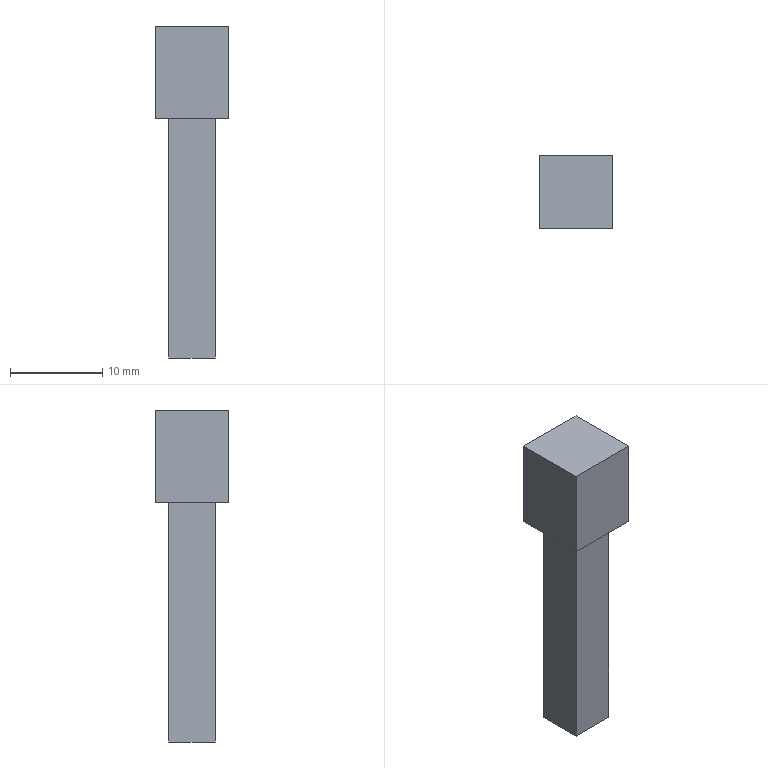Part | NX | features DATUM_CSYS 3, EXTRUDE 2, SKETCH 2 | 1 solid | 11 faces | box 8 x 8 x 36 mm | volume 1290 mm3 | plane 11
STEP:
#1=CARTESIAN_POINT('',(0.,5.,0.));
#2=VERTEX_POINT('',#1);
#3=CARTESIAN_POINT('',(0.,0.,0.));
#4=VERTEX_POINT('',#3);
#5=CARTESIAN_POINT('',(0.,5.,0.));
#6=DIRECTION('',(0.,-1.,0.));
#7=VECTOR('',#6,1000.);
#8=LINE('',#5,#7);
#9=EDGE_CURVE('',#2,#4,#8,.T.);
#10=ORIENTED_EDGE('',*,*,#9,.T.);
#11=CARTESIAN_POINT('',(0.,0.,26.));
#12=VERTEX_POINT('',#11);
#13=CARTESIAN_POINT('',(0.,0.,26.));
#14=DIRECTION('',(0.,0.,-1.));
#15=VECTOR('',#14,1000.);
#16=LINE('',#13,#15);
#17=EDGE_CURVE('',#12,#4,#16,.T.);
#18=ORIENTED_EDGE('',*,*,#17,.F.);
#19=CARTESIAN_POINT('',(0.,5.,26.));
#20=VERTEX_POINT('',#19);
#21=CARTESIAN_POINT('',(0.,5.,26.));
#22=DIRECTION('',(0.,-1.,0.));
#23=VECTOR('',#22,1000.);
#24=LINE('',#21,#23);
#25=EDGE_CURVE('',#20,#12,#24,.T.);
#26=ORIENTED_EDGE('',*,*,#25,.F.);
#27=CARTESIAN_POINT('',(0.,5.,26.));
#28=DIRECTION('',(0.,0.,-1.));
#29=VECTOR('',#28,1000.);
#30=LINE('',#27,#29);
#31=EDGE_CURVE('',#20,#2,#30,.T.);
#32=ORIENTED_EDGE('',*,*,#31,.T.);
#33=EDGE_LOOP('',(#10,#18,#26,#32));
#34=FACE_BOUND('',#33,.T.);
#35=CARTESIAN_POINT('',(0.,5.,26.));
#36=DIRECTION('',(1.,0.,0.));
#37=DIRECTION('',(0.,1.,0.));
#38=AXIS2_PLACEMENT_3D('',#35,#36,#37);
#39=PLANE('',#38);
#40=ADVANCED_FACE('',(#34),#39,.F.);
#41=CARTESIAN_POINT('',(5.,0.,0.));
#42=VERTEX_POINT('',#41);
#43=CARTESIAN_POINT('',(0.,0.,0.));
#44=DIRECTION('',(1.,0.,0.));
#45=VECTOR('',#44,1000.);
#46=LINE('',#43,#45);
#47=EDGE_CURVE('',#4,#42,#46,.T.);
#48=ORIENTED_EDGE('',*,*,#47,.T.);
#49=CARTESIAN_POINT('',(5.,0.,26.));
#50=VERTEX_POINT('',#49);
#51=CARTESIAN_POINT('',(5.,0.,26.));
#52=DIRECTION('',(0.,0.,-1.));
#53=VECTOR('',#52,1000.);
#54=LINE('',#51,#53);
#55=EDGE_CURVE('',#50,#42,#54,.T.);
#56=ORIENTED_EDGE('',*,*,#55,.F.);
#57=CARTESIAN_POINT('',(0.,0.,26.));
#58=DIRECTION('',(1.,0.,0.));
#59=VECTOR('',#58,1000.);
#60=LINE('',#57,#59);
#61=EDGE_CURVE('',#12,#50,#60,.T.);
#62=ORIENTED_EDGE('',*,*,#61,.F.);
#63=ORIENTED_EDGE('',*,*,#17,.T.);
#64=EDGE_LOOP('',(#48,#56,#62,#63));
#65=FACE_BOUND('',#64,.T.);
#66=CARTESIAN_POINT('',(0.,0.,26.));
#67=DIRECTION('',(0.,1.,0.));
#68=DIRECTION('',(0.,0.,1.));
#69=AXIS2_PLACEMENT_3D('',#66,#67,#68);
#70=PLANE('',#69);
#71=ADVANCED_FACE('',(#65),#70,.F.);
#72=CARTESIAN_POINT('',(5.,5.,0.));
#73=VERTEX_POINT('',#72);
#74=CARTESIAN_POINT('',(5.,0.,0.));
#75=DIRECTION('',(0.,1.,0.));
#76=VECTOR('',#75,1000.);
#77=LINE('',#74,#76);
#78=EDGE_CURVE('',#42,#73,#77,.T.);
#79=ORIENTED_EDGE('',*,*,#78,.T.);
#80=CARTESIAN_POINT('',(5.,5.,26.));
#81=VERTEX_POINT('',#80);
#82=CARTESIAN_POINT('',(5.,5.,26.));
#83=DIRECTION('',(0.,0.,-1.));
#84=VECTOR('',#83,1000.);
#85=LINE('',#82,#84);
#86=EDGE_CURVE('',#81,#73,#85,.T.);
#87=ORIENTED_EDGE('',*,*,#86,.F.);
#88=CARTESIAN_POINT('',(5.,0.,26.));
#89=DIRECTION('',(0.,1.,0.));
#90=VECTOR('',#89,1000.);
#91=LINE('',#88,#90);
#92=EDGE_CURVE('',#50,#81,#91,.T.);
#93=ORIENTED_EDGE('',*,*,#92,.F.);
#94=ORIENTED_EDGE('',*,*,#55,.T.);
#95=EDGE_LOOP('',(#79,#87,#93,#94));
#96=FACE_BOUND('',#95,.T.);
#97=CARTESIAN_POINT('',(5.,0.,26.));
#98=DIRECTION('',(-1.,0.,0.));
#99=DIRECTION('',(0.,0.,1.));
#100=AXIS2_PLACEMENT_3D('',#97,#98,#99);
#101=PLANE('',#100);
#102=ADVANCED_FACE('',(#96),#101,.F.);
#103=CARTESIAN_POINT('',(5.,5.,0.));
#104=DIRECTION('',(-1.,0.,0.));
#105=VECTOR('',#104,1000.);
#106=LINE('',#103,#105);
#107=EDGE_CURVE('',#73,#2,#106,.T.);
#108=ORIENTED_EDGE('',*,*,#107,.T.);
#109=ORIENTED_EDGE('',*,*,#31,.F.);
#110=CARTESIAN_POINT('',(5.,5.,26.));
#111=DIRECTION('',(-1.,0.,0.));
#112=VECTOR('',#111,1000.);
#113=LINE('',#110,#112);
#114=EDGE_CURVE('',#81,#20,#113,.T.);
#115=ORIENTED_EDGE('',*,*,#114,.F.);
#116=ORIENTED_EDGE('',*,*,#86,.T.);
#117=EDGE_LOOP('',(#108,#109,#115,#116));
#118=FACE_BOUND('',#117,.T.);
#119=CARTESIAN_POINT('',(5.,5.,26.));
#120=DIRECTION('',(0.,-1.,0.));
#121=DIRECTION('',(0.,0.,-1.));
#122=AXIS2_PLACEMENT_3D('',#119,#120,#121);
#123=PLANE('',#122);
#124=ADVANCED_FACE('',(#118),#123,.F.);
#125=ORIENTED_EDGE('',*,*,#9,.F.);
#126=ORIENTED_EDGE('',*,*,#107,.F.);
#127=ORIENTED_EDGE('',*,*,#78,.F.);
#128=ORIENTED_EDGE('',*,*,#47,.F.);
#129=EDGE_LOOP('',(#125,#126,#127,#128));
#130=FACE_BOUND('',#129,.T.);
#131=CARTESIAN_POINT('',(0.,0.,0.));
#132=DIRECTION('',(0.,0.,1.));
#133=DIRECTION('',(1.,0.,0.));
#134=AXIS2_PLACEMENT_3D('',#131,#132,#133);
#135=PLANE('',#134);
#136=ADVANCED_FACE('',(#130),#135,.F.);
#137=CARTESIAN_POINT('',(-1.5,6.5,26.));
#138=VERTEX_POINT('',#137);
#139=CARTESIAN_POINT('',(-1.5,-1.5,26.));
#140=VERTEX_POINT('',#139);
#141=CARTESIAN_POINT('',(-1.5,6.5,26.));
#142=DIRECTION('',(0.,-1.,0.));
#143=VECTOR('',#142,1000.);
#144=LINE('',#141,#143);
#145=EDGE_CURVE('',#138,#140,#144,.T.);
#146=ORIENTED_EDGE('',*,*,#145,.F.);
#147=CARTESIAN_POINT('',(6.5,6.5,26.));
#148=VERTEX_POINT('',#147);
#149=CARTESIAN_POINT('',(6.5,6.5,26.));
#150=DIRECTION('',(-1.,0.,0.));
#151=VECTOR('',#150,1000.);
#152=LINE('',#149,#151);
#153=EDGE_CURVE('',#148,#138,#152,.T.);
#154=ORIENTED_EDGE('',*,*,#153,.F.);
#155=CARTESIAN_POINT('',(6.5,-1.5,26.));
#156=VERTEX_POINT('',#155);
#157=CARTESIAN_POINT('',(6.5,-1.5,26.));
#158=DIRECTION('',(0.,1.,0.));
#159=VECTOR('',#158,1000.);
#160=LINE('',#157,#159);
#161=EDGE_CURVE('',#156,#148,#160,.T.);
#162=ORIENTED_EDGE('',*,*,#161,.F.);
#163=CARTESIAN_POINT('',(-1.5,-1.5,26.));
#164=DIRECTION('',(1.,0.,0.));
#165=VECTOR('',#164,1000.);
#166=LINE('',#163,#165);
#167=EDGE_CURVE('',#140,#156,#166,.T.);
#168=ORIENTED_EDGE('',*,*,#167,.F.);
#169=EDGE_LOOP('',(#146,#154,#162,#168));
#170=FACE_BOUND('',#169,.T.);
#171=ORIENTED_EDGE('',*,*,#114,.T.);
#172=ORIENTED_EDGE('',*,*,#25,.T.);
#173=ORIENTED_EDGE('',*,*,#61,.T.);
#174=ORIENTED_EDGE('',*,*,#92,.T.);
#175=EDGE_LOOP('',(#171,#172,#173,#174));
#176=FACE_BOUND('',#175,.T.);
#177=CARTESIAN_POINT('',(0.,0.,26.));
#178=DIRECTION('',(0.,0.,1.));
#179=DIRECTION('',(1.,0.,0.));
#180=AXIS2_PLACEMENT_3D('',#177,#178,#179);
#181=PLANE('',#180);
#182=ADVANCED_FACE('',(#170,#176),#181,.F.);
#183=ORIENTED_EDGE('',*,*,#145,.T.);
#184=CARTESIAN_POINT('',(-1.5,-1.5,36.));
#185=VERTEX_POINT('',#184);
#186=CARTESIAN_POINT('',(-1.5,-1.5,36.));
#187=DIRECTION('',(0.,0.,-1.));
#188=VECTOR('',#187,1000.);
#189=LINE('',#186,#188);
#190=EDGE_CURVE('',#185,#140,#189,.T.);
#191=ORIENTED_EDGE('',*,*,#190,.F.);
#192=CARTESIAN_POINT('',(-1.5,6.5,36.));
#193=VERTEX_POINT('',#192);
#194=CARTESIAN_POINT('',(-1.5,6.5,36.));
#195=DIRECTION('',(0.,-1.,0.));
#196=VECTOR('',#195,1000.);
#197=LINE('',#194,#196);
#198=EDGE_CURVE('',#193,#185,#197,.T.);
#199=ORIENTED_EDGE('',*,*,#198,.F.);
#200=CARTESIAN_POINT('',(-1.5,6.5,36.));
#201=DIRECTION('',(0.,0.,-1.));
#202=VECTOR('',#201,1000.);
#203=LINE('',#200,#202);
#204=EDGE_CURVE('',#193,#138,#203,.T.);
#205=ORIENTED_EDGE('',*,*,#204,.T.);
#206=EDGE_LOOP('',(#183,#191,#199,#205));
#207=FACE_BOUND('',#206,.T.);
#208=CARTESIAN_POINT('',(-1.5,6.5,36.));
#209=DIRECTION('',(1.,0.,0.));
#210=DIRECTION('',(0.,0.,-1.));
#211=AXIS2_PLACEMENT_3D('',#208,#209,#210);
#212=PLANE('',#211);
#213=ADVANCED_FACE('',(#207),#212,.F.);
#214=ORIENTED_EDGE('',*,*,#167,.T.);
#215=CARTESIAN_POINT('',(6.5,-1.5,36.));
#216=VERTEX_POINT('',#215);
#217=CARTESIAN_POINT('',(6.5,-1.5,36.));
#218=DIRECTION('',(0.,0.,-1.));
#219=VECTOR('',#218,1000.);
#220=LINE('',#217,#219);
#221=EDGE_CURVE('',#216,#156,#220,.T.);
#222=ORIENTED_EDGE('',*,*,#221,.F.);
#223=CARTESIAN_POINT('',(-1.5,-1.5,36.));
#224=DIRECTION('',(1.,0.,0.));
#225=VECTOR('',#224,1000.);
#226=LINE('',#223,#225);
#227=EDGE_CURVE('',#185,#216,#226,.T.);
#228=ORIENTED_EDGE('',*,*,#227,.F.);
#229=ORIENTED_EDGE('',*,*,#190,.T.);
#230=EDGE_LOOP('',(#214,#222,#228,#229));
#231=FACE_BOUND('',#230,.T.);
#232=CARTESIAN_POINT('',(-1.5,-1.5,36.));
#233=DIRECTION('',(0.,1.,0.));
#234=DIRECTION('',(0.,0.,1.));
#235=AXIS2_PLACEMENT_3D('',#232,#233,#234);
#236=PLANE('',#235);
#237=ADVANCED_FACE('',(#231),#236,.F.);
#238=ORIENTED_EDGE('',*,*,#161,.T.);
#239=CARTESIAN_POINT('',(6.5,6.5,36.));
#240=VERTEX_POINT('',#239);
#241=CARTESIAN_POINT('',(6.5,6.5,36.));
#242=DIRECTION('',(0.,0.,-1.));
#243=VECTOR('',#242,1000.);
#244=LINE('',#241,#243);
#245=EDGE_CURVE('',#240,#148,#244,.T.);
#246=ORIENTED_EDGE('',*,*,#245,.F.);
#247=CARTESIAN_POINT('',(6.5,-1.5,36.));
#248=DIRECTION('',(0.,1.,0.));
#249=VECTOR('',#248,1000.);
#250=LINE('',#247,#249);
#251=EDGE_CURVE('',#216,#240,#250,.T.);
#252=ORIENTED_EDGE('',*,*,#251,.F.);
#253=ORIENTED_EDGE('',*,*,#221,.T.);
#254=EDGE_LOOP('',(#238,#246,#252,#253));
#255=FACE_BOUND('',#254,.T.);
#256=CARTESIAN_POINT('',(6.5,-1.5,36.));
#257=DIRECTION('',(-1.,0.,0.));
#258=DIRECTION('',(0.,0.,1.));
#259=AXIS2_PLACEMENT_3D('',#256,#257,#258);
#260=PLANE('',#259);
#261=ADVANCED_FACE('',(#255),#260,.F.);
#262=ORIENTED_EDGE('',*,*,#153,.T.);
#263=ORIENTED_EDGE('',*,*,#204,.F.);
#264=CARTESIAN_POINT('',(6.5,6.5,36.));
#265=DIRECTION('',(-1.,0.,0.));
#266=VECTOR('',#265,1000.);
#267=LINE('',#264,#266);
#268=EDGE_CURVE('',#240,#193,#267,.T.);
#269=ORIENTED_EDGE('',*,*,#268,.F.);
#270=ORIENTED_EDGE('',*,*,#245,.T.);
#271=EDGE_LOOP('',(#262,#263,#269,#270));
#272=FACE_BOUND('',#271,.T.);
#273=CARTESIAN_POINT('',(6.5,6.5,36.));
#274=DIRECTION('',(0.,-1.,0.));
#275=DIRECTION('',(0.,0.,-1.));
#276=AXIS2_PLACEMENT_3D('',#273,#274,#275);
#277=PLANE('',#276);
#278=ADVANCED_FACE('',(#272),#277,.F.);
#279=ORIENTED_EDGE('',*,*,#198,.T.);
#280=ORIENTED_EDGE('',*,*,#227,.T.);
#281=ORIENTED_EDGE('',*,*,#251,.T.);
#282=ORIENTED_EDGE('',*,*,#268,.T.);
#283=EDGE_LOOP('',(#279,#280,#281,#282));
#284=FACE_BOUND('',#283,.T.);
#285=CARTESIAN_POINT('',(0.,0.,36.));
#286=DIRECTION('',(0.,0.,1.));
#287=DIRECTION('',(1.,0.,0.));
#288=AXIS2_PLACEMENT_3D('',#285,#286,#287);
#289=PLANE('',#288);
#290=ADVANCED_FACE('',(#284),#289,.T.);
#291=CLOSED_SHELL('',(#40,#71,#102,#124,#136,#182,#213,#237,#261,#278,#290));
#292=MANIFOLD_SOLID_BREP('',#291);
#293=(LENGTH_UNIT()NAMED_UNIT(*)SI_UNIT(.MILLI.,.METRE.));
#294=UNCERTAINTY_MEASURE_WITH_UNIT(LENGTH_MEASURE(0.00001),#293,'','');
#295=(NAMED_UNIT(*)PLANE_ANGLE_UNIT()SI_UNIT($,.RADIAN.));
#296=(NAMED_UNIT(*)SI_UNIT($,.STERADIAN.)SOLID_ANGLE_UNIT());
#297=(GEOMETRIC_REPRESENTATION_CONTEXT(3)GLOBAL_UNCERTAINTY_ASSIGNED_CONTEXT((#294))GLOBAL_UNIT_ASSIGNED_CONTEXT((#293,#295,#296))REPRESENTATION_CONTEXT('',''));
#298=ADVANCED_BREP_SHAPE_REPRESENTATION('',(#292),#297);